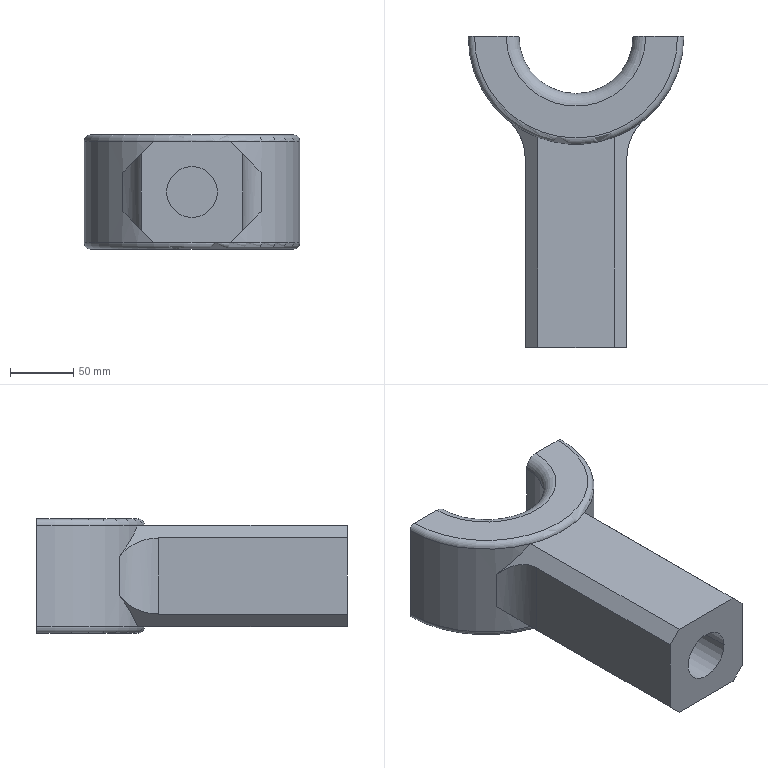Part | Creo | features CURVE 3, CUT 3, DATUM PLANE 3, ROUND 3, CHAMFER 1, COORDINATE SYSTEM 1, MIRROR 1, PROTRUSION 1 | 1 solid | 25 faces | box 170 x 245 x 90 mm | volume 1592709 mm3 | plane 14 | cylinder 7 | torus 4 | commonest cylinder face diameters 40 x2 80 x2 170 x2 90 x1
STEP:
#1=CARTESIAN_POINT('',(0.,0.,0.));
#2=DIRECTION('',(0.,0.,1.));
#3=DIRECTION('',(1.,0.,0.));
#4=AXIS2_PLACEMENT_3D('',#1,#2,#3);
#5=CARTESIAN_POINT('',(80.,245.,-45.));
#6=VERTEX_POINT('',#5);
#7=CARTESIAN_POINT('',(-80.,245.,-45.));
#8=VERTEX_POINT('',#7);
#9=CARTESIAN_POINT('',(0.,245.,-45.));
#10=DIRECTION('',(0.,0.,-1.));
#11=DIRECTION('',(1.,0.,0.));
#12=AXIS2_PLACEMENT_3D('',#9,#10,#11);
#13=CIRCLE('',#12,80.);
#14=EDGE_CURVE('',#6,#8,#13,.T.);
#15=ORIENTED_EDGE('',*,*,#14,.F.);
#16=CARTESIAN_POINT('',(55.,245.,-45.));
#17=VERTEX_POINT('',#16);
#18=CARTESIAN_POINT('',(80.,245.,-45.));
#19=DIRECTION('',(-1.,0.,0.));
#20=VECTOR('',#19,25.);
#21=LINE('',#18,#20);
#22=EDGE_CURVE('',#6,#17,#21,.T.);
#23=ORIENTED_EDGE('',*,*,#22,.T.);
#24=CARTESIAN_POINT('',(-55.,245.,-45.));
#25=VERTEX_POINT('',#24);
#26=CARTESIAN_POINT('',(0.,245.,-45.));
#27=DIRECTION('',(0.,0.,1.));
#28=DIRECTION('',(-1.,0.,0.));
#29=AXIS2_PLACEMENT_3D('',#26,#27,#28);
#30=CIRCLE('',#29,55.);
#31=EDGE_CURVE('',#25,#17,#30,.T.);
#32=ORIENTED_EDGE('',*,*,#31,.F.);
#33=CARTESIAN_POINT('',(-55.,245.,-45.));
#34=DIRECTION('',(-1.,0.,0.));
#35=VECTOR('',#34,25.);
#36=LINE('',#33,#35);
#37=EDGE_CURVE('',#25,#8,#36,.T.);
#38=ORIENTED_EDGE('',*,*,#37,.T.);
#39=EDGE_LOOP('',(#15,#23,#32,#38));
#40=FACE_OUTER_BOUND('',#39,.F.);
#41=CARTESIAN_POINT('',(0.,0.,-45.));
#42=DIRECTION('',(0.,0.,1.));
#43=DIRECTION('',(1.,0.,0.));
#44=AXIS2_PLACEMENT_3D('',#41,#42,#43);
#45=PLANE('',#44);
#46=ADVANCED_FACE('',(#40),#45,.F.);
#47=CARTESIAN_POINT('',(-30.,165.47,-40.));
#48=VERTEX_POINT('',#47);
#49=CARTESIAN_POINT('',(30.,165.47,-40.));
#50=VERTEX_POINT('',#49);
#51=CARTESIAN_POINT('',(0.,245.,-40.));
#52=DIRECTION('',(0.,0.,1.));
#53=DIRECTION('',(-0.3529,-0.9356,0.));
#54=AXIS2_PLACEMENT_3D('',#51,#52,#53);
#55=CIRCLE('',#54,85.);
#56=EDGE_CURVE('',#48,#50,#55,.T.);
#57=ORIENTED_EDGE('',*,*,#56,.T.);
#58=CARTESIAN_POINT('',(85.,245.,-40.));
#59=VERTEX_POINT('',#58);
#60=CARTESIAN_POINT('',(0.,245.,-40.));
#61=DIRECTION('',(0.,0.,1.));
#62=DIRECTION('',(0.3529,-0.9356,0.));
#63=AXIS2_PLACEMENT_3D('',#60,#61,#62);
#64=CIRCLE('',#63,85.);
#65=EDGE_CURVE('',#50,#59,#64,.T.);
#66=ORIENTED_EDGE('',*,*,#65,.T.);
#67=CARTESIAN_POINT('',(80.,245.,-40.));
#68=DIRECTION('',(0.,1.,0.));
#69=DIRECTION('',(1.,0.,0.));
#70=AXIS2_PLACEMENT_3D('',#67,#68,#69);
#71=CIRCLE('',#70,5.);
#72=EDGE_CURVE('',#59,#6,#71,.T.);
#73=ORIENTED_EDGE('',*,*,#72,.T.);
#74=ORIENTED_EDGE('',*,*,#14,.T.);
#75=CARTESIAN_POINT('',(-85.,245.,-40.));
#76=VERTEX_POINT('',#75);
#77=CARTESIAN_POINT('',(-80.,245.,-40.));
#78=DIRECTION('',(0.,1.,0.));
#79=DIRECTION('',(0.,0.,-1.));
#80=AXIS2_PLACEMENT_3D('',#77,#78,#79);
#81=CIRCLE('',#80,5.);
#82=EDGE_CURVE('',#8,#76,#81,.T.);
#83=ORIENTED_EDGE('',*,*,#82,.T.);
#84=CARTESIAN_POINT('',(0.,245.,-40.));
#85=DIRECTION('',(0.,0.,1.));
#86=DIRECTION('',(-1.,0.,0.));
#87=AXIS2_PLACEMENT_3D('',#84,#85,#86);
#88=CIRCLE('',#87,85.);
#89=EDGE_CURVE('',#76,#48,#88,.T.);
#90=ORIENTED_EDGE('',*,*,#89,.T.);
#91=EDGE_LOOP('',(#57,#66,#73,#74,#83,#90));
#92=FACE_OUTER_BOUND('',#91,.F.);
#93=CARTESIAN_POINT('',(0.,245.,-40.));
#94=DIRECTION('',(0.,0.,1.));
#95=DIRECTION('',(-0.0009333,1.,0.));
#96=AXIS2_PLACEMENT_3D('',#93,#94,#95);
#97=TOROIDAL_SURFACE('',#96,80.,5.);
#98=ADVANCED_FACE('',(#92),#97,.T.);
#99=ORIENTED_EDGE('',*,*,#56,.F.);
#100=CARTESIAN_POINT('',(-30.,0.,-40.));
#101=VERTEX_POINT('',#100);
#102=CARTESIAN_POINT('',(-30.,165.47,-40.));
#103=DIRECTION('',(0.,-1.,0.));
#104=VECTOR('',#103,165.47);
#105=LINE('',#102,#104);
#106=EDGE_CURVE('',#48,#101,#105,.T.);
#107=ORIENTED_EDGE('',*,*,#106,.T.);
#108=CARTESIAN_POINT('',(30.,0.,-40.));
#109=VERTEX_POINT('',#108);
#110=CARTESIAN_POINT('',(-30.,0.,-40.));
#111=DIRECTION('',(1.,0.,0.));
#112=VECTOR('',#111,60.);
#113=LINE('',#110,#112);
#114=EDGE_CURVE('',#101,#109,#113,.T.);
#115=ORIENTED_EDGE('',*,*,#114,.T.);
#116=CARTESIAN_POINT('',(30.,0.,-40.));
#117=DIRECTION('',(0.,1.,0.));
#118=VECTOR('',#117,165.47);
#119=LINE('',#116,#118);
#120=EDGE_CURVE('',#109,#50,#119,.T.);
#121=ORIENTED_EDGE('',*,*,#120,.T.);
#122=EDGE_LOOP('',(#99,#107,#115,#121));
#123=FACE_OUTER_BOUND('',#122,.F.);
#124=CARTESIAN_POINT('',(0.,0.,-40.));
#125=DIRECTION('',(0.,0.,1.));
#126=DIRECTION('',(1.,0.,0.));
#127=AXIS2_PLACEMENT_3D('',#124,#125,#126);
#128=PLANE('',#127);
#129=ADVANCED_FACE('',(#123),#128,.F.);
#130=ORIENTED_EDGE('',*,*,#106,.F.);
#131=CARTESIAN_POINT('',(-54.4,179.688,-15.6));
#132=VERTEX_POINT('',#131);
#133=CARTESIAN_POINT('',(-30.,165.47,-40.));
#134=CARTESIAN_POINT('',(-38.578,168.706,-31.422));
#135=CARTESIAN_POINT('',(-46.75,173.316,-23.25));
#136=CARTESIAN_POINT('',(-54.4,179.688,-15.6));
#137=B_SPLINE_CURVE_WITH_KNOTS('',3,(#133,#134,#135,#136),.UNSPECIFIED.,.F.,.F.,(4,4),(0.,1.),.UNSPECIFIED.);
#138=EDGE_CURVE('',#48,#132,#137,.T.);
#139=ORIENTED_EDGE('',*,*,#138,.T.);
#140=CARTESIAN_POINT('',(-40.,148.953,-30.));
#141=VERTEX_POINT('',#140);
#142=CARTESIAN_POINT('',(-40.,148.953,-30.));
#143=CARTESIAN_POINT('',(-40.,152.484,-30.));
#144=CARTESIAN_POINT('',(-40.892,158.826,-29.108));
#145=CARTESIAN_POINT('',(-44.973,169.652,-25.027));
#146=CARTESIAN_POINT('',(-50.097,176.104,-19.903));
#147=CARTESIAN_POINT('',(-54.4,179.688,-15.6));
#148=B_SPLINE_CURVE_WITH_KNOTS('',3,(#142,#143,#144,#145,#146,#147),.UNSPECIFIED.,.F.,.F.,(4,1,1,4),(0.,0.25,0.5,1.),.UNSPECIFIED.);
#149=EDGE_CURVE('',#141,#132,#148,.T.);
#150=ORIENTED_EDGE('',*,*,#149,.F.);
#151=CARTESIAN_POINT('',(-40.,0.,-30.));
#152=VERTEX_POINT('',#151);
#153=CARTESIAN_POINT('',(-40.,148.953,-30.));
#154=DIRECTION('',(0.,-1.,0.));
#155=VECTOR('',#154,148.953);
#156=LINE('',#153,#155);
#157=EDGE_CURVE('',#141,#152,#156,.T.);
#158=ORIENTED_EDGE('',*,*,#157,.T.);
#159=CARTESIAN_POINT('',(-40.,0.,-30.));
#160=DIRECTION('',(0.7071,0.,-0.7071));
#161=VECTOR('',#160,14.142);
#162=LINE('',#159,#161);
#163=EDGE_CURVE('',#152,#101,#162,.T.);
#164=ORIENTED_EDGE('',*,*,#163,.T.);
#165=EDGE_LOOP('',(#130,#139,#150,#158,#164));
#166=FACE_OUTER_BOUND('',#165,.F.);
#167=CARTESIAN_POINT('',(-35.,82.735,-35.));
#168=DIRECTION('',(-0.7071,0.,-0.7071));
#169=DIRECTION('',(0.7071,0.,-0.7071));
#170=AXIS2_PLACEMENT_3D('',#167,#168,#169);
#171=PLANE('',#170);
#172=ADVANCED_FACE('',(#166),#171,.T.);
#173=CARTESIAN_POINT('',(-30.,165.47,40.));
#174=VERTEX_POINT('',#173);
#175=CARTESIAN_POINT('',(-85.,245.,40.));
#176=VERTEX_POINT('',#175);
#177=CARTESIAN_POINT('',(0.,245.,40.));
#178=DIRECTION('',(0.,0.,-1.));
#179=DIRECTION('',(-0.3529,-0.9356,0.));
#180=AXIS2_PLACEMENT_3D('',#177,#178,#179);
#181=CIRCLE('',#180,85.);
#182=EDGE_CURVE('',#174,#176,#181,.T.);
#183=ORIENTED_EDGE('',*,*,#182,.F.);
#184=CARTESIAN_POINT('',(-54.4,179.688,15.6));
#185=VERTEX_POINT('',#184);
#186=CARTESIAN_POINT('',(-54.4,179.688,15.6));
#187=CARTESIAN_POINT('',(-46.75,173.316,23.25));
#188=CARTESIAN_POINT('',(-38.578,168.706,31.422));
#189=CARTESIAN_POINT('',(-30.,165.47,40.));
#190=B_SPLINE_CURVE_WITH_KNOTS('',3,(#186,#187,#188,#189),.UNSPECIFIED.,.F.,.F.,(4,4),(0.,1.),.UNSPECIFIED.);
#191=EDGE_CURVE('',#185,#174,#190,.T.);
#192=ORIENTED_EDGE('',*,*,#191,.F.);
#193=CARTESIAN_POINT('',(-54.4,179.688,-15.6));
#194=DIRECTION('',(0.,0.,1.));
#195=VECTOR('',#194,31.2);
#196=LINE('',#193,#195);
#197=EDGE_CURVE('',#132,#185,#196,.T.);
#198=ORIENTED_EDGE('',*,*,#197,.F.);
#199=ORIENTED_EDGE('',*,*,#138,.F.);
#200=ORIENTED_EDGE('',*,*,#89,.F.);
#201=CARTESIAN_POINT('',(-85.,245.,-40.));
#202=DIRECTION('',(0.,0.,1.));
#203=VECTOR('',#202,80.);
#204=LINE('',#201,#203);
#205=EDGE_CURVE('',#76,#176,#204,.T.);
#206=ORIENTED_EDGE('',*,*,#205,.T.);
#207=EDGE_LOOP('',(#183,#192,#198,#199,#200,#206));
#208=FACE_OUTER_BOUND('',#207,.F.);
#209=CARTESIAN_POINT('',(0.,245.,-45.));
#210=DIRECTION('',(0.,0.,1.));
#211=DIRECTION('',(1.,0.,0.));
#212=AXIS2_PLACEMENT_3D('',#209,#210,#211);
#213=CYLINDRICAL_SURFACE('',#212,85.);
#214=ADVANCED_FACE('',(#208),#213,.T.);
#215=CARTESIAN_POINT('',(85.,245.,40.));
#216=VERTEX_POINT('',#215);
#217=CARTESIAN_POINT('',(30.,165.47,40.));
#218=VERTEX_POINT('',#217);
#219=CARTESIAN_POINT('',(0.,245.,40.));
#220=DIRECTION('',(0.,0.,-1.));
#221=DIRECTION('',(1.,0.,0.));
#222=AXIS2_PLACEMENT_3D('',#219,#220,#221);
#223=CIRCLE('',#222,85.);
#224=EDGE_CURVE('',#216,#218,#223,.T.);
#225=ORIENTED_EDGE('',*,*,#224,.F.);
#226=CARTESIAN_POINT('',(85.,245.,-40.));
#227=DIRECTION('',(0.,0.,1.));
#228=VECTOR('',#227,80.);
#229=LINE('',#226,#228);
#230=EDGE_CURVE('',#59,#216,#229,.T.);
#231=ORIENTED_EDGE('',*,*,#230,.F.);
#232=ORIENTED_EDGE('',*,*,#65,.F.);
#233=CARTESIAN_POINT('',(54.4,179.688,-15.6));
#234=VERTEX_POINT('',#233);
#235=CARTESIAN_POINT('',(54.4,179.688,-15.6));
#236=CARTESIAN_POINT('',(46.75,173.316,-23.25));
#237=CARTESIAN_POINT('',(38.578,168.706,-31.422));
#238=CARTESIAN_POINT('',(30.,165.47,-40.));
#239=B_SPLINE_CURVE_WITH_KNOTS('',3,(#235,#236,#237,#238),.UNSPECIFIED.,.F.,.F.,(4,4),(0.,1.),.UNSPECIFIED.);
#240=EDGE_CURVE('',#234,#50,#239,.T.);
#241=ORIENTED_EDGE('',*,*,#240,.F.);
#242=CARTESIAN_POINT('',(54.4,179.688,15.6));
#243=VERTEX_POINT('',#242);
#244=CARTESIAN_POINT('',(54.4,179.688,-15.6));
#245=DIRECTION('',(0.,0.,1.));
#246=VECTOR('',#245,31.2);
#247=LINE('',#244,#246);
#248=EDGE_CURVE('',#234,#243,#247,.T.);
#249=ORIENTED_EDGE('',*,*,#248,.T.);
#250=CARTESIAN_POINT('',(30.,165.47,40.));
#251=CARTESIAN_POINT('',(38.578,168.706,31.422));
#252=CARTESIAN_POINT('',(46.75,173.316,23.25));
#253=CARTESIAN_POINT('',(54.4,179.688,15.6));
#254=B_SPLINE_CURVE_WITH_KNOTS('',3,(#250,#251,#252,#253),.UNSPECIFIED.,.F.,.F.,(4,4),(0.,1.),.UNSPECIFIED.);
#255=EDGE_CURVE('',#218,#243,#254,.T.);
#256=ORIENTED_EDGE('',*,*,#255,.F.);
#257=EDGE_LOOP('',(#225,#231,#232,#241,#249,#256));
#258=FACE_OUTER_BOUND('',#257,.F.);
#259=CARTESIAN_POINT('',(0.,245.,-45.));
#260=DIRECTION('',(0.,0.,1.));
#261=DIRECTION('',(1.,0.,0.));
#262=AXIS2_PLACEMENT_3D('',#259,#260,#261);
#263=CYLINDRICAL_SURFACE('',#262,85.);
#264=ADVANCED_FACE('',(#258),#263,.T.);
#265=CARTESIAN_POINT('',(0.,245.,40.));
#266=DIRECTION('',(0.,0.,-1.));
#267=DIRECTION('',(0.3529,-0.9356,0.));
#268=AXIS2_PLACEMENT_3D('',#265,#266,#267);
#269=CIRCLE('',#268,85.);
#270=EDGE_CURVE('',#218,#174,#269,.T.);
#271=ORIENTED_EDGE('',*,*,#270,.T.);
#272=ORIENTED_EDGE('',*,*,#182,.T.);
#273=CARTESIAN_POINT('',(-80.,245.,45.));
#274=VERTEX_POINT('',#273);
#275=CARTESIAN_POINT('',(-80.,245.,40.));
#276=DIRECTION('',(0.,1.,0.));
#277=DIRECTION('',(-1.,0.,0.));
#278=AXIS2_PLACEMENT_3D('',#275,#276,#277);
#279=CIRCLE('',#278,5.);
#280=EDGE_CURVE('',#176,#274,#279,.T.);
#281=ORIENTED_EDGE('',*,*,#280,.T.);
#282=CARTESIAN_POINT('',(80.,245.,45.));
#283=VERTEX_POINT('',#282);
#284=CARTESIAN_POINT('',(0.,245.,45.));
#285=DIRECTION('',(0.,0.,1.));
#286=DIRECTION('',(-1.,0.,0.));
#287=AXIS2_PLACEMENT_3D('',#284,#285,#286);
#288=CIRCLE('',#287,80.);
#289=EDGE_CURVE('',#274,#283,#288,.T.);
#290=ORIENTED_EDGE('',*,*,#289,.T.);
#291=CARTESIAN_POINT('',(80.,245.,40.));
#292=DIRECTION('',(0.,1.,0.));
#293=DIRECTION('',(0.,0.,1.));
#294=AXIS2_PLACEMENT_3D('',#291,#292,#293);
#295=CIRCLE('',#294,5.);
#296=EDGE_CURVE('',#283,#216,#295,.T.);
#297=ORIENTED_EDGE('',*,*,#296,.T.);
#298=ORIENTED_EDGE('',*,*,#224,.T.);
#299=EDGE_LOOP('',(#271,#272,#281,#290,#297,#298));
#300=FACE_OUTER_BOUND('',#299,.F.);
#301=CARTESIAN_POINT('',(0.,245.,40.));
#302=DIRECTION('',(0.,0.,1.));
#303=DIRECTION('',(0.001088,1.,0.));
#304=AXIS2_PLACEMENT_3D('',#301,#302,#303);
#305=TOROIDAL_SURFACE('',#304,80.,5.);
#306=ADVANCED_FACE('',(#300),#305,.T.);
#307=ORIENTED_EDGE('',*,*,#270,.F.);
#308=CARTESIAN_POINT('',(30.,0.,40.));
#309=VERTEX_POINT('',#308);
#310=CARTESIAN_POINT('',(30.,165.47,40.));
#311=DIRECTION('',(0.,-1.,0.));
#312=VECTOR('',#311,165.47);
#313=LINE('',#310,#312);
#314=EDGE_CURVE('',#218,#309,#313,.T.);
#315=ORIENTED_EDGE('',*,*,#314,.T.);
#316=CARTESIAN_POINT('',(-30.,0.,40.));
#317=VERTEX_POINT('',#316);
#318=CARTESIAN_POINT('',(-30.,0.,40.));
#319=DIRECTION('',(1.,0.,0.));
#320=VECTOR('',#319,60.);
#321=LINE('',#318,#320);
#322=EDGE_CURVE('',#317,#309,#321,.T.);
#323=ORIENTED_EDGE('',*,*,#322,.F.);
#324=CARTESIAN_POINT('',(-30.,0.,40.));
#325=DIRECTION('',(0.,1.,0.));
#326=VECTOR('',#325,165.47);
#327=LINE('',#324,#326);
#328=EDGE_CURVE('',#317,#174,#327,.T.);
#329=ORIENTED_EDGE('',*,*,#328,.T.);
#330=EDGE_LOOP('',(#307,#315,#323,#329));
#331=FACE_OUTER_BOUND('',#330,.F.);
#332=CARTESIAN_POINT('',(0.,0.,40.));
#333=DIRECTION('',(0.,0.,1.));
#334=DIRECTION('',(1.,0.,0.));
#335=AXIS2_PLACEMENT_3D('',#332,#333,#334);
#336=PLANE('',#335);
#337=ADVANCED_FACE('',(#331),#336,.T.);
#338=ORIENTED_EDGE('',*,*,#314,.F.);
#339=ORIENTED_EDGE('',*,*,#255,.T.);
#340=CARTESIAN_POINT('',(40.,148.953,30.));
#341=VERTEX_POINT('',#340);
#342=CARTESIAN_POINT('',(40.,148.953,30.));
#343=CARTESIAN_POINT('',(40.,152.484,30.));
#344=CARTESIAN_POINT('',(40.892,158.826,29.108));
#345=CARTESIAN_POINT('',(44.973,169.652,25.027));
#346=CARTESIAN_POINT('',(50.097,176.104,19.903));
#347=CARTESIAN_POINT('',(54.4,179.688,15.6));
#348=B_SPLINE_CURVE_WITH_KNOTS('',3,(#342,#343,#344,#345,#346,#347),.UNSPECIFIED.,.F.,.F.,(4,1,1,4),(0.,0.25,0.5,1.),.UNSPECIFIED.);
#349=EDGE_CURVE('',#341,#243,#348,.T.);
#350=ORIENTED_EDGE('',*,*,#349,.F.);
#351=CARTESIAN_POINT('',(40.,0.,30.));
#352=VERTEX_POINT('',#351);
#353=CARTESIAN_POINT('',(40.,148.953,30.));
#354=DIRECTION('',(0.,-1.,0.));
#355=VECTOR('',#354,148.953);
#356=LINE('',#353,#355);
#357=EDGE_CURVE('',#341,#352,#356,.T.);
#358=ORIENTED_EDGE('',*,*,#357,.T.);
#359=CARTESIAN_POINT('',(40.,0.,30.));
#360=DIRECTION('',(-0.7071,0.,0.7071));
#361=VECTOR('',#360,14.142);
#362=LINE('',#359,#361);
#363=EDGE_CURVE('',#352,#309,#362,.T.);
#364=ORIENTED_EDGE('',*,*,#363,.T.);
#365=EDGE_LOOP('',(#338,#339,#350,#358,#364));
#366=FACE_OUTER_BOUND('',#365,.F.);
#367=CARTESIAN_POINT('',(35.,82.735,35.));
#368=DIRECTION('',(0.7071,0.,0.7071));
#369=DIRECTION('',(-0.7071,0.,0.7071));
#370=AXIS2_PLACEMENT_3D('',#367,#368,#369);
#371=PLANE('',#370);
#372=ADVANCED_FACE('',(#366),#371,.T.);
#373=ORIENTED_EDGE('',*,*,#248,.F.);
#374=CARTESIAN_POINT('',(40.,148.953,-30.));
#375=VERTEX_POINT('',#374);
#376=CARTESIAN_POINT('',(54.4,179.688,-15.6));
#377=CARTESIAN_POINT('',(50.097,176.104,-19.903));
#378=CARTESIAN_POINT('',(44.973,169.652,-25.027));
#379=CARTESIAN_POINT('',(40.892,158.826,-29.108));
#380=CARTESIAN_POINT('',(40.,152.484,-30.));
#381=CARTESIAN_POINT('',(40.,148.953,-30.));
#382=B_SPLINE_CURVE_WITH_KNOTS('',3,(#376,#377,#378,#379,#380,#381),.UNSPECIFIED.,.F.,.F.,(4,1,1,4),(0.,0.5,0.75,1.),.UNSPECIFIED.);
#383=EDGE_CURVE('',#234,#375,#382,.T.);
#384=ORIENTED_EDGE('',*,*,#383,.T.);
#385=CARTESIAN_POINT('',(40.,148.953,-30.));
#386=DIRECTION('',(0.,0.,1.));
#387=VECTOR('',#386,60.);
#388=LINE('',#385,#387);
#389=EDGE_CURVE('',#375,#341,#388,.T.);
#390=ORIENTED_EDGE('',*,*,#389,.T.);
#391=ORIENTED_EDGE('',*,*,#349,.T.);
#392=EDGE_LOOP('',(#373,#384,#390,#391));
#393=FACE_OUTER_BOUND('',#392,.F.);
#394=CARTESIAN_POINT('',(80.,148.953,-162.324));
#395=DIRECTION('',(0.,0.,1.));
#396=DIRECTION('',(-0.64,0.7684,0.));
#397=AXIS2_PLACEMENT_3D('',#394,#395,#396);
#398=CYLINDRICAL_SURFACE('',#397,40.);
#399=ADVANCED_FACE('',(#393),#398,.F.);
#400=ORIENTED_EDGE('',*,*,#120,.F.);
#401=CARTESIAN_POINT('',(40.,0.,-30.));
#402=VERTEX_POINT('',#401);
#403=CARTESIAN_POINT('',(30.,0.,-40.));
#404=DIRECTION('',(0.7071,0.,0.7071));
#405=VECTOR('',#404,14.142);
#406=LINE('',#403,#405);
#407=EDGE_CURVE('',#109,#402,#406,.T.);
#408=ORIENTED_EDGE('',*,*,#407,.T.);
#409=CARTESIAN_POINT('',(40.,0.,-30.));
#410=DIRECTION('',(0.,1.,0.));
#411=VECTOR('',#410,148.953);
#412=LINE('',#409,#411);
#413=EDGE_CURVE('',#402,#375,#412,.T.);
#414=ORIENTED_EDGE('',*,*,#413,.T.);
#415=ORIENTED_EDGE('',*,*,#383,.F.);
#416=ORIENTED_EDGE('',*,*,#240,.T.);
#417=EDGE_LOOP('',(#400,#408,#414,#415,#416));
#418=FACE_OUTER_BOUND('',#417,.F.);
#419=CARTESIAN_POINT('',(35.,82.735,-35.));
#420=DIRECTION('',(0.7071,0.,-0.7071));
#421=DIRECTION('',(-0.7071,0.,-0.7071));
#422=AXIS2_PLACEMENT_3D('',#419,#420,#421);
#423=PLANE('',#422);
#424=ADVANCED_FACE('',(#418),#423,.T.);
#425=CARTESIAN_POINT('',(-40.,0.,30.));
#426=VERTEX_POINT('',#425);
#427=CARTESIAN_POINT('',(-30.,0.,40.));
#428=DIRECTION('',(-0.7071,0.,-0.7071));
#429=VECTOR('',#428,14.142);
#430=LINE('',#427,#429);
#431=EDGE_CURVE('',#317,#426,#430,.T.);
#432=ORIENTED_EDGE('',*,*,#431,.F.);
#433=ORIENTED_EDGE('',*,*,#322,.T.);
#434=ORIENTED_EDGE('',*,*,#363,.F.);
#435=CARTESIAN_POINT('',(40.,0.,-30.));
#436=DIRECTION('',(0.,0.,1.));
#437=VECTOR('',#436,60.);
#438=LINE('',#435,#437);
#439=EDGE_CURVE('',#402,#352,#438,.T.);
#440=ORIENTED_EDGE('',*,*,#439,.F.);
#441=ORIENTED_EDGE('',*,*,#407,.F.);
#442=ORIENTED_EDGE('',*,*,#114,.F.);
#443=ORIENTED_EDGE('',*,*,#163,.F.);
#444=CARTESIAN_POINT('',(-40.,0.,-30.));
#445=DIRECTION('',(0.,0.,1.));
#446=VECTOR('',#445,60.);
#447=LINE('',#444,#446);
#448=EDGE_CURVE('',#152,#426,#447,.T.);
#449=ORIENTED_EDGE('',*,*,#448,.T.);
#450=EDGE_LOOP('',(#432,#433,#434,#440,#441,#442,#443,#449));
#451=FACE_OUTER_BOUND('',#450,.F.);
#452=CARTESIAN_POINT('',(20.,0.,0.));
#453=VERTEX_POINT('',#452);
#454=CARTESIAN_POINT('',(-20.,0.,0.));
#455=VERTEX_POINT('',#454);
#456=CARTESIAN_POINT('',(0.,0.,0.));
#457=DIRECTION('',(0.,-1.,0.));
#458=DIRECTION('',(1.,0.,0.));
#459=AXIS2_PLACEMENT_3D('',#456,#457,#458);
#460=CIRCLE('',#459,20.);
#461=EDGE_CURVE('',#453,#455,#460,.T.);
#462=ORIENTED_EDGE('',*,*,#461,.T.);
#463=CARTESIAN_POINT('',(0.,0.,0.));
#464=DIRECTION('',(0.,-1.,0.));
#465=DIRECTION('',(-1.,0.,0.));
#466=AXIS2_PLACEMENT_3D('',#463,#464,#465);
#467=CIRCLE('',#466,20.);
#468=EDGE_CURVE('',#455,#453,#467,.T.);
#469=ORIENTED_EDGE('',*,*,#468,.T.);
#470=EDGE_LOOP('',(#462,#469));
#471=FACE_BOUND('',#470,.F.);
#472=CARTESIAN_POINT('',(-40.,0.,-45.));
#473=DIRECTION('',(0.,-1.,0.));
#474=DIRECTION('',(1.,0.,0.));
#475=AXIS2_PLACEMENT_3D('',#472,#473,#474);
#476=PLANE('',#475);
#477=ADVANCED_FACE('',(#451,#471),#476,.T.);
#478=ORIENTED_EDGE('',*,*,#328,.F.);
#479=ORIENTED_EDGE('',*,*,#431,.T.);
#480=CARTESIAN_POINT('',(-40.,148.953,30.));
#481=VERTEX_POINT('',#480);
#482=CARTESIAN_POINT('',(-40.,0.,30.));
#483=DIRECTION('',(0.,1.,0.));
#484=VECTOR('',#483,148.953);
#485=LINE('',#482,#484);
#486=EDGE_CURVE('',#426,#481,#485,.T.);
#487=ORIENTED_EDGE('',*,*,#486,.T.);
#488=CARTESIAN_POINT('',(-54.4,179.688,15.6));
#489=CARTESIAN_POINT('',(-50.097,176.104,19.903));
#490=CARTESIAN_POINT('',(-44.973,169.652,25.027));
#491=CARTESIAN_POINT('',(-40.892,158.826,29.108));
#492=CARTESIAN_POINT('',(-40.,152.484,30.));
#493=CARTESIAN_POINT('',(-40.,148.953,30.));
#494=B_SPLINE_CURVE_WITH_KNOTS('',3,(#488,#489,#490,#491,#492,#493),.UNSPECIFIED.,.F.,.F.,(4,1,1,4),(0.,0.5,0.75,1.),.UNSPECIFIED.);
#495=EDGE_CURVE('',#185,#481,#494,.T.);
#496=ORIENTED_EDGE('',*,*,#495,.F.);
#497=ORIENTED_EDGE('',*,*,#191,.T.);
#498=EDGE_LOOP('',(#478,#479,#487,#496,#497));
#499=FACE_OUTER_BOUND('',#498,.F.);
#500=CARTESIAN_POINT('',(-35.,82.735,35.));
#501=DIRECTION('',(-0.7071,0.,0.7071));
#502=DIRECTION('',(0.7071,0.,0.7071));
#503=AXIS2_PLACEMENT_3D('',#500,#501,#502);
#504=PLANE('',#503);
#505=ADVANCED_FACE('',(#499),#504,.T.);
#506=CARTESIAN_POINT('',(-40.,148.953,-30.));
#507=DIRECTION('',(0.,0.,1.));
#508=VECTOR('',#507,60.);
#509=LINE('',#506,#508);
#510=EDGE_CURVE('',#141,#481,#509,.T.);
#511=ORIENTED_EDGE('',*,*,#510,.T.);
#512=ORIENTED_EDGE('',*,*,#486,.F.);
#513=ORIENTED_EDGE('',*,*,#448,.F.);
#514=ORIENTED_EDGE('',*,*,#157,.F.);
#515=EDGE_LOOP('',(#511,#512,#513,#514));
#516=FACE_OUTER_BOUND('',#515,.F.);
#517=CARTESIAN_POINT('',(-40.,170.,-45.));
#518=DIRECTION('',(-1.,0.,0.));
#519=DIRECTION('',(0.,-1.,0.));
#520=AXIS2_PLACEMENT_3D('',#517,#518,#519);
#521=PLANE('',#520);
#522=ADVANCED_FACE('',(#516),#521,.T.);
#523=ORIENTED_EDGE('',*,*,#510,.F.);
#524=ORIENTED_EDGE('',*,*,#149,.T.);
#525=ORIENTED_EDGE('',*,*,#197,.T.);
#526=ORIENTED_EDGE('',*,*,#495,.T.);
#527=EDGE_LOOP('',(#523,#524,#525,#526));
#528=FACE_OUTER_BOUND('',#527,.F.);
#529=CARTESIAN_POINT('',(-80.,148.953,-162.324));
#530=DIRECTION('',(0.,0.,1.));
#531=DIRECTION('',(1.,0.,0.));
#532=AXIS2_PLACEMENT_3D('',#529,#530,#531);
#533=CYLINDRICAL_SURFACE('',#532,40.);
#534=ADVANCED_FACE('',(#528),#533,.F.);
#535=ORIENTED_EDGE('',*,*,#389,.F.);
#536=ORIENTED_EDGE('',*,*,#413,.F.);
#537=ORIENTED_EDGE('',*,*,#439,.T.);
#538=ORIENTED_EDGE('',*,*,#357,.F.);
#539=EDGE_LOOP('',(#535,#536,#537,#538));
#540=FACE_OUTER_BOUND('',#539,.F.);
#541=CARTESIAN_POINT('',(40.,0.,-45.));
#542=DIRECTION('',(1.,0.,0.));
#543=DIRECTION('',(0.,1.,0.));
#544=AXIS2_PLACEMENT_3D('',#541,#542,#543);
#545=PLANE('',#544);
#546=ADVANCED_FACE('',(#540),#545,.T.);
#547=ORIENTED_EDGE('',*,*,#461,.F.);
#548=CARTESIAN_POINT('',(20.,120.,0.));
#549=VERTEX_POINT('',#548);
#550=CARTESIAN_POINT('',(20.,0.,0.));
#551=DIRECTION('',(0.,1.,0.));
#552=VECTOR('',#551,120.);
#553=LINE('',#550,#552);
#554=EDGE_CURVE('',#453,#549,#553,.T.);
#555=ORIENTED_EDGE('',*,*,#554,.T.);
#556=CARTESIAN_POINT('',(-20.,120.,0.));
#557=VERTEX_POINT('',#556);
#558=CARTESIAN_POINT('',(0.,120.,0.));
#559=DIRECTION('',(0.,-1.,0.));
#560=DIRECTION('',(1.,0.,0.));
#561=AXIS2_PLACEMENT_3D('',#558,#559,#560);
#562=CIRCLE('',#561,20.);
#563=EDGE_CURVE('',#549,#557,#562,.T.);
#564=ORIENTED_EDGE('',*,*,#563,.T.);
#565=CARTESIAN_POINT('',(-20.,0.,0.));
#566=DIRECTION('',(0.,1.,0.));
#567=VECTOR('',#566,120.);
#568=LINE('',#565,#567);
#569=EDGE_CURVE('',#455,#557,#568,.T.);
#570=ORIENTED_EDGE('',*,*,#569,.F.);
#571=EDGE_LOOP('',(#547,#555,#564,#570));
#572=FACE_OUTER_BOUND('',#571,.F.);
#573=CARTESIAN_POINT('',(0.,0.,0.));
#574=DIRECTION('',(0.,-1.,0.));
#575=DIRECTION('',(1.,0.,0.));
#576=AXIS2_PLACEMENT_3D('',#573,#574,#575);
#577=CYLINDRICAL_SURFACE('',#576,20.);
#578=ADVANCED_FACE('',(#572),#577,.F.);
#579=ORIENTED_EDGE('',*,*,#468,.F.);
#580=ORIENTED_EDGE('',*,*,#569,.T.);
#581=CARTESIAN_POINT('',(0.,120.,0.));
#582=DIRECTION('',(0.,-1.,0.));
#583=DIRECTION('',(-1.,0.,0.));
#584=AXIS2_PLACEMENT_3D('',#581,#582,#583);
#585=CIRCLE('',#584,20.);
#586=EDGE_CURVE('',#557,#549,#585,.T.);
#587=ORIENTED_EDGE('',*,*,#586,.T.);
#588=ORIENTED_EDGE('',*,*,#554,.F.);
#589=EDGE_LOOP('',(#579,#580,#587,#588));
#590=FACE_OUTER_BOUND('',#589,.F.);
#591=CARTESIAN_POINT('',(0.,0.,0.));
#592=DIRECTION('',(0.,-1.,0.));
#593=DIRECTION('',(1.,0.,0.));
#594=AXIS2_PLACEMENT_3D('',#591,#592,#593);
#595=CYLINDRICAL_SURFACE('',#594,20.);
#596=ADVANCED_FACE('',(#590),#595,.F.);
#597=ORIENTED_EDGE('',*,*,#563,.F.);
#598=ORIENTED_EDGE('',*,*,#586,.F.);
#599=EDGE_LOOP('',(#597,#598));
#600=FACE_OUTER_BOUND('',#599,.F.);
#601=CARTESIAN_POINT('',(0.,120.,-45.));
#602=DIRECTION('',(0.,-1.,0.));
#603=DIRECTION('',(1.,0.,0.));
#604=AXIS2_PLACEMENT_3D('',#601,#602,#603);
#605=PLANE('',#604);
#606=ADVANCED_FACE('',(#600),#605,.T.);
#607=ORIENTED_EDGE('',*,*,#280,.F.);
#608=ORIENTED_EDGE('',*,*,#205,.F.);
#609=ORIENTED_EDGE('',*,*,#82,.F.);
#610=ORIENTED_EDGE('',*,*,#37,.F.);
#611=CARTESIAN_POINT('',(-45.,245.,-35.));
#612=VERTEX_POINT('',#611);
#613=CARTESIAN_POINT('',(-55.,245.,-35.));
#614=DIRECTION('',(0.,1.,0.));
#615=DIRECTION('',(1.,0.,0.));
#616=AXIS2_PLACEMENT_3D('',#613,#614,#615);
#617=CIRCLE('',#616,10.);
#618=EDGE_CURVE('',#612,#25,#617,.T.);
#619=ORIENTED_EDGE('',*,*,#618,.F.);
#620=CARTESIAN_POINT('',(-45.,245.,35.));
#621=VERTEX_POINT('',#620);
#622=CARTESIAN_POINT('',(-45.,245.,-35.));
#623=DIRECTION('',(0.,0.,1.));
#624=VECTOR('',#623,70.);
#625=LINE('',#622,#624);
#626=EDGE_CURVE('',#612,#621,#625,.T.);
#627=ORIENTED_EDGE('',*,*,#626,.T.);
#628=CARTESIAN_POINT('',(-55.,245.,45.));
#629=VERTEX_POINT('',#628);
#630=CARTESIAN_POINT('',(-55.,245.,35.));
#631=DIRECTION('',(0.,1.,0.));
#632=DIRECTION('',(0.,0.,1.));
#633=AXIS2_PLACEMENT_3D('',#630,#631,#632);
#634=CIRCLE('',#633,10.);
#635=EDGE_CURVE('',#629,#621,#634,.T.);
#636=ORIENTED_EDGE('',*,*,#635,.F.);
#637=CARTESIAN_POINT('',(-55.,245.,45.));
#638=DIRECTION('',(-1.,0.,0.));
#639=VECTOR('',#638,25.);
#640=LINE('',#637,#639);
#641=EDGE_CURVE('',#629,#274,#640,.T.);
#642=ORIENTED_EDGE('',*,*,#641,.T.);
#643=EDGE_LOOP('',(#607,#608,#609,#610,#619,#627,#636,#642));
#644=FACE_OUTER_BOUND('',#643,.F.);
#645=CARTESIAN_POINT('',(-45.,245.,-45.));
#646=DIRECTION('',(0.,1.,0.));
#647=DIRECTION('',(-1.,0.,0.));
#648=AXIS2_PLACEMENT_3D('',#645,#646,#647);
#649=PLANE('',#648);
#650=ADVANCED_FACE('',(#644),#649,.T.);
#651=ORIENTED_EDGE('',*,*,#31,.T.);
#652=CARTESIAN_POINT('',(45.,245.,-35.));
#653=VERTEX_POINT('',#652);
#654=CARTESIAN_POINT('',(55.,245.,-35.));
#655=DIRECTION('',(0.,1.,0.));
#656=DIRECTION('',(0.,0.,-1.));
#657=AXIS2_PLACEMENT_3D('',#654,#655,#656);
#658=CIRCLE('',#657,10.);
#659=EDGE_CURVE('',#17,#653,#658,.T.);
#660=ORIENTED_EDGE('',*,*,#659,.T.);
#661=CARTESIAN_POINT('',(0.,245.,-35.));
#662=DIRECTION('',(0.,0.,-1.));
#663=DIRECTION('',(1.,0.,0.));
#664=AXIS2_PLACEMENT_3D('',#661,#662,#663);
#665=CIRCLE('',#664,45.);
#666=EDGE_CURVE('',#653,#612,#665,.T.);
#667=ORIENTED_EDGE('',*,*,#666,.T.);
#668=ORIENTED_EDGE('',*,*,#618,.T.);
#669=EDGE_LOOP('',(#651,#660,#667,#668));
#670=FACE_OUTER_BOUND('',#669,.F.);
#671=CARTESIAN_POINT('',(0.,245.,-35.));
#672=DIRECTION('',(0.,0.,1.));
#673=DIRECTION('',(-0.001486,1.,0.));
#674=AXIS2_PLACEMENT_3D('',#671,#672,#673);
#675=TOROIDAL_SURFACE('',#674,55.,10.);
#676=ADVANCED_FACE('',(#670),#675,.T.);
#677=ORIENTED_EDGE('',*,*,#296,.F.);
#678=CARTESIAN_POINT('',(55.,245.,45.));
#679=VERTEX_POINT('',#678);
#680=CARTESIAN_POINT('',(80.,245.,45.));
#681=DIRECTION('',(-1.,0.,0.));
#682=VECTOR('',#681,25.);
#683=LINE('',#680,#682);
#684=EDGE_CURVE('',#283,#679,#683,.T.);
#685=ORIENTED_EDGE('',*,*,#684,.T.);
#686=CARTESIAN_POINT('',(45.,245.,35.));
#687=VERTEX_POINT('',#686);
#688=CARTESIAN_POINT('',(55.,245.,35.));
#689=DIRECTION('',(0.,1.,0.));
#690=DIRECTION('',(-1.,0.,0.));
#691=AXIS2_PLACEMENT_3D('',#688,#689,#690);
#692=CIRCLE('',#691,10.);
#693=EDGE_CURVE('',#687,#679,#692,.T.);
#694=ORIENTED_EDGE('',*,*,#693,.F.);
#695=CARTESIAN_POINT('',(45.,245.,-35.));
#696=DIRECTION('',(0.,0.,1.));
#697=VECTOR('',#696,70.);
#698=LINE('',#695,#697);
#699=EDGE_CURVE('',#653,#687,#698,.T.);
#700=ORIENTED_EDGE('',*,*,#699,.F.);
#701=ORIENTED_EDGE('',*,*,#659,.F.);
#702=ORIENTED_EDGE('',*,*,#22,.F.);
#703=ORIENTED_EDGE('',*,*,#72,.F.);
#704=ORIENTED_EDGE('',*,*,#230,.T.);
#705=EDGE_LOOP('',(#677,#685,#694,#700,#701,#702,#703,#704));
#706=FACE_OUTER_BOUND('',#705,.F.);
#707=CARTESIAN_POINT('',(85.,245.,-45.));
#708=DIRECTION('',(0.,1.,0.));
#709=DIRECTION('',(-1.,0.,0.));
#710=AXIS2_PLACEMENT_3D('',#707,#708,#709);
#711=PLANE('',#710);
#712=ADVANCED_FACE('',(#706),#711,.T.);
#713=ORIENTED_EDGE('',*,*,#289,.F.);
#714=ORIENTED_EDGE('',*,*,#641,.F.);
#715=CARTESIAN_POINT('',(0.,245.,45.));
#716=DIRECTION('',(0.,0.,-1.));
#717=DIRECTION('',(1.,0.,0.));
#718=AXIS2_PLACEMENT_3D('',#715,#716,#717);
#719=CIRCLE('',#718,55.);
#720=EDGE_CURVE('',#679,#629,#719,.T.);
#721=ORIENTED_EDGE('',*,*,#720,.F.);
#722=ORIENTED_EDGE('',*,*,#684,.F.);
#723=EDGE_LOOP('',(#713,#714,#721,#722));
#724=FACE_OUTER_BOUND('',#723,.F.);
#725=CARTESIAN_POINT('',(0.,0.,45.));
#726=DIRECTION('',(0.,0.,1.));
#727=DIRECTION('',(1.,0.,0.));
#728=AXIS2_PLACEMENT_3D('',#725,#726,#727);
#729=PLANE('',#728);
#730=ADVANCED_FACE('',(#724),#729,.T.);
#731=ORIENTED_EDGE('',*,*,#720,.T.);
#732=ORIENTED_EDGE('',*,*,#635,.T.);
#733=CARTESIAN_POINT('',(0.,245.,35.));
#734=DIRECTION('',(0.,0.,1.));
#735=DIRECTION('',(-1.,0.,0.));
#736=AXIS2_PLACEMENT_3D('',#733,#734,#735);
#737=CIRCLE('',#736,45.);
#738=EDGE_CURVE('',#621,#687,#737,.T.);
#739=ORIENTED_EDGE('',*,*,#738,.T.);
#740=ORIENTED_EDGE('',*,*,#693,.T.);
#741=EDGE_LOOP('',(#731,#732,#739,#740));
#742=FACE_OUTER_BOUND('',#741,.F.);
#743=CARTESIAN_POINT('',(0.,245.,35.));
#744=DIRECTION('',(0.,0.,1.));
#745=DIRECTION('',(0.0009333,1.,0.));
#746=AXIS2_PLACEMENT_3D('',#743,#744,#745);
#747=TOROIDAL_SURFACE('',#746,55.,10.);
#748=ADVANCED_FACE('',(#742),#747,.T.);
#749=ORIENTED_EDGE('',*,*,#738,.F.);
#750=ORIENTED_EDGE('',*,*,#626,.F.);
#751=ORIENTED_EDGE('',*,*,#666,.F.);
#752=ORIENTED_EDGE('',*,*,#699,.T.);
#753=EDGE_LOOP('',(#749,#750,#751,#752));
#754=FACE_OUTER_BOUND('',#753,.F.);
#755=CARTESIAN_POINT('',(0.,245.,-45.));
#756=DIRECTION('',(0.,0.,1.));
#757=DIRECTION('',(1.,0.,0.));
#758=AXIS2_PLACEMENT_3D('',#755,#756,#757);
#759=CYLINDRICAL_SURFACE('',#758,45.);
#760=ADVANCED_FACE('',(#754),#759,.F.);
#761=CLOSED_SHELL('',(#46,#98,#129,#172,#214,#264,#306,#337,#372,#399,#424,#477,#505,#522,#534,#546,#578,#596,#606,#650,#676,#712,#730,#748,#760));
#762=MANIFOLD_SOLID_BREP('',#761);
#763=(LENGTH_UNIT()NAMED_UNIT(*)SI_UNIT(.MILLI.,.METRE.));
#764=UNCERTAINTY_MEASURE_WITH_UNIT(LENGTH_MEASURE(0.03115),#763,'','');
#765=(NAMED_UNIT(*)PLANE_ANGLE_UNIT()SI_UNIT($,.RADIAN.));
#766=PLANE_ANGLE_MEASURE_WITH_UNIT(PLANE_ANGLE_MEASURE(0.01745),#765);
#767=(CONVERSION_BASED_UNIT('DEGREE',#766)NAMED_UNIT(*)PLANE_ANGLE_UNIT());
#768=(NAMED_UNIT(*)SI_UNIT($,.STERADIAN.)SOLID_ANGLE_UNIT());
#769=(GEOMETRIC_REPRESENTATION_CONTEXT(3)GLOBAL_UNCERTAINTY_ASSIGNED_CONTEXT((#764))GLOBAL_UNIT_ASSIGNED_CONTEXT((#763,#767,#768))REPRESENTATION_CONTEXT('',''));
#770=ADVANCED_BREP_SHAPE_REPRESENTATION('',(#4,#762),#769);